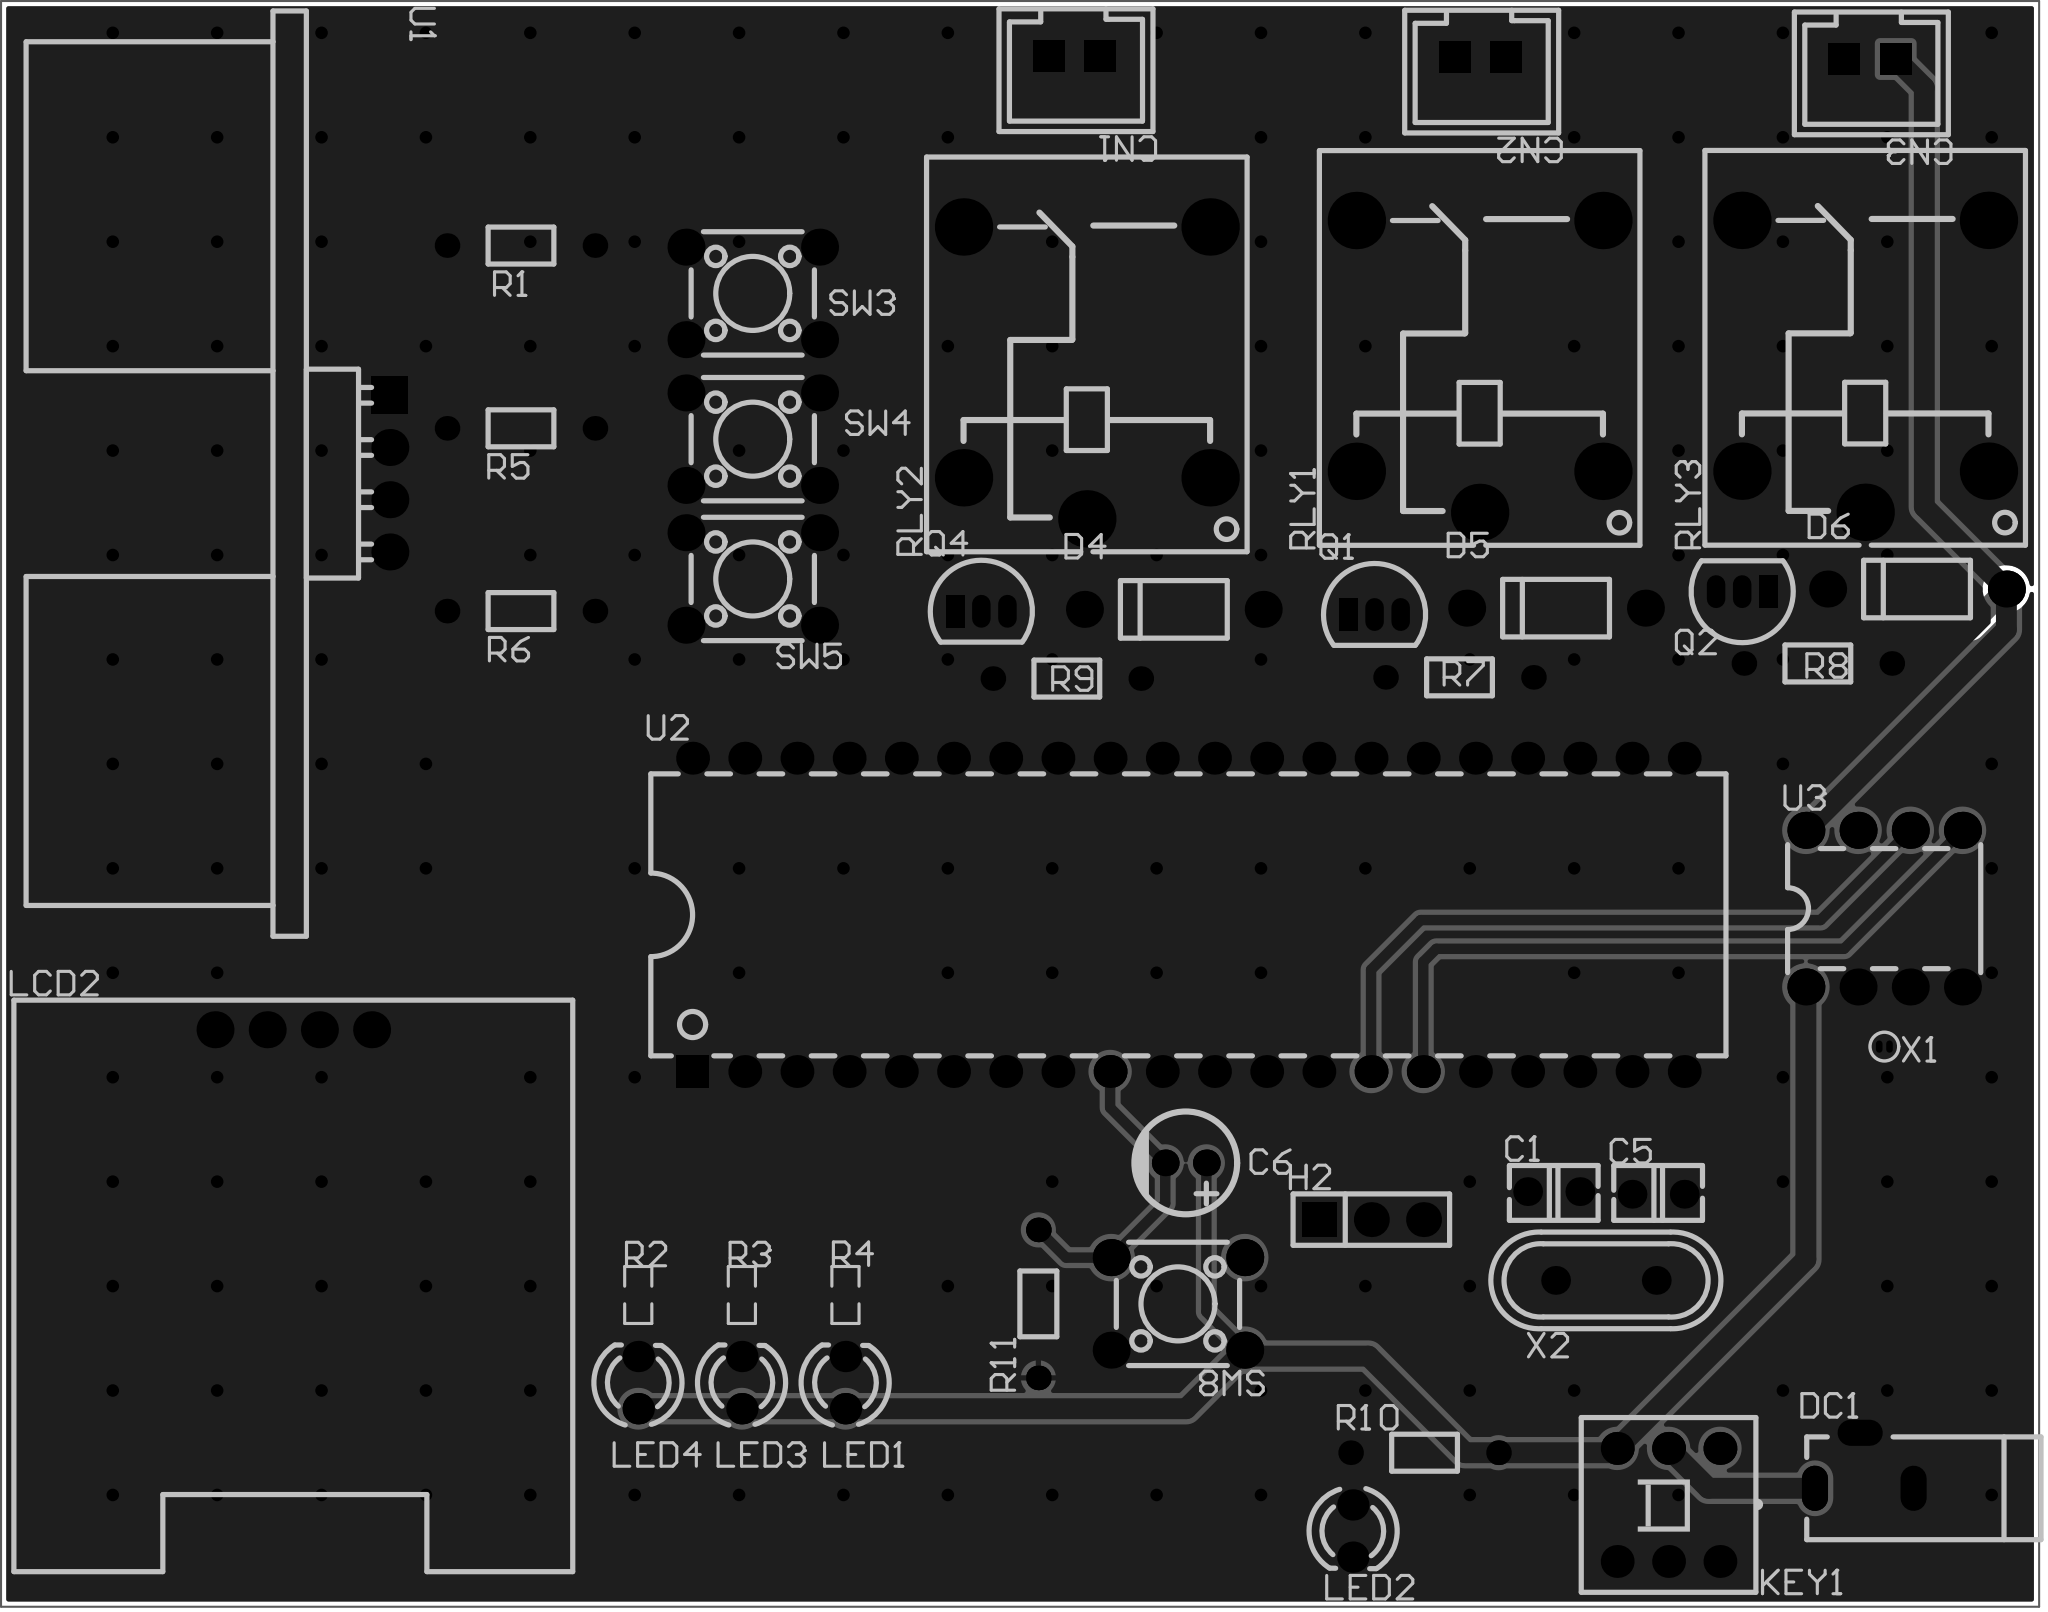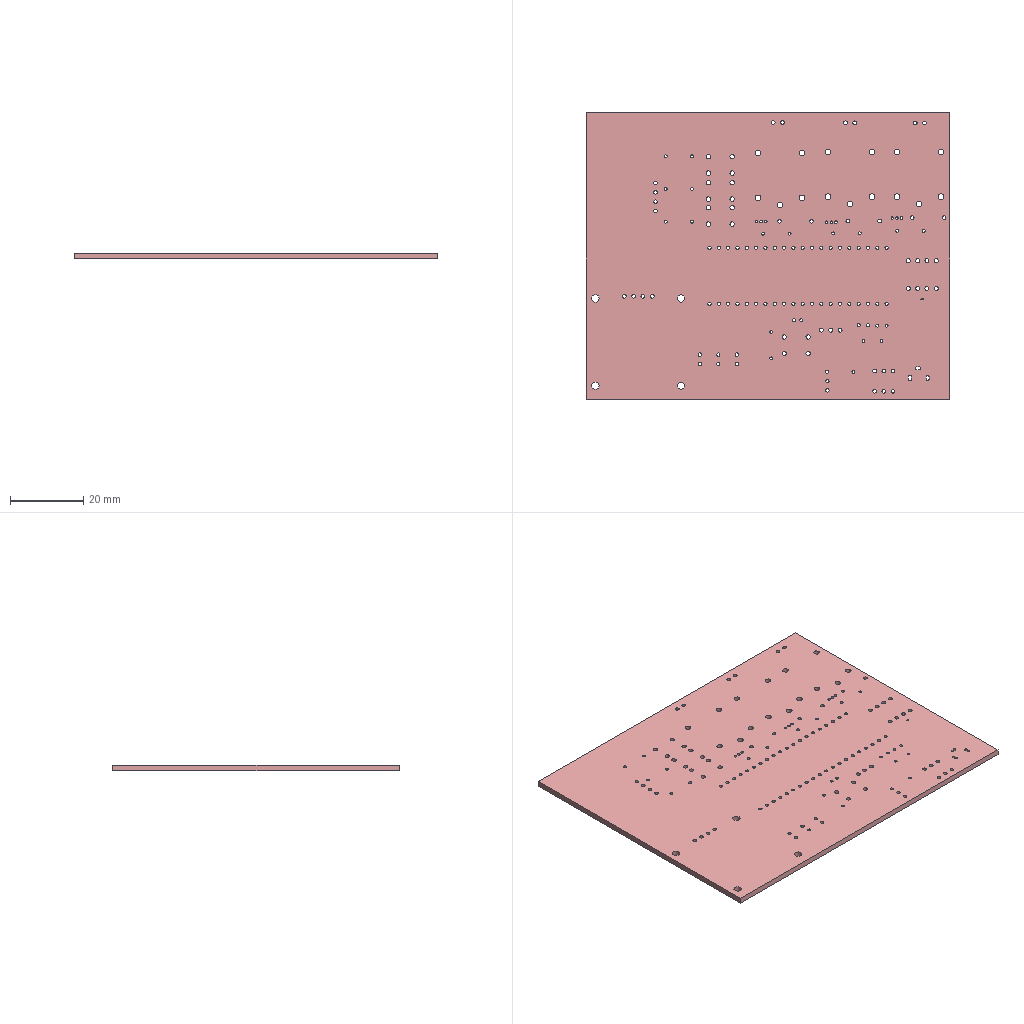Circuit board layout | Altium Designer | box 99.2 x 78.1 x 1.6 mm
Layer stack:
# Altium Designer layer stack of  (unit mm; dielectric type: 0 none, 1 core, 2 prepreg, 3 surface material)
index,name,kind,layer,copper_thickness_mm,dielectric_type,dielectric_thickness_mm,dielectric_material,dielectric_constant
0,Top Paste Mask Layer,other,,,,,,
1,Top Silkscreen Layer,other,,,,,,
2,Top Solder Mask Layer,dielectric,,,3,0.01,,3.3
3,Top Layer,copper,Top Layer,0.035,,,,
4,Dielectric1,dielectric,,,3,1.51,FR4,4.5
5,Bottom Layer,copper,Bottom Layer,0.035,,,,
6,Bottom Solder Mask Layer,dielectric,,,3,0.01,,3.3
7,Bottom Silkscreen Layer,other,,,,,,
8,Bottom Paste Mask Layer,other,,,,,,
# drill layer pairs: low layer,high layer
drill_pair,Top Layer,Bottom Layer
Part placement:
Designator,Comment,Layer,Footprint,Center-X(mm),Center-Y(mm),Rotation
C1,30pF,TopLayer,CAP-TH_L3.8-W2.5-P2.54-D0.50,161.671,110.49,0
C5,30pF,TopLayer,CAP-TH_L3.8-W2.5-P2.54-D0.50,166.751,110.363,180
CN1,XH2.54-2PIN-直针,TopLayer,CONN-TH_XH2.54-2P,138.356,165.735,180
CN2,XH2.54-2PIN-直针,TopLayer,CONN-TH_XH2.54-2P,158.101,165.668,180
CN3,XH2.54-2PIN-直针,TopLayer,CONN-TH_XH2.54-2P,177.064,165.582,180
D4,,TopLayer,DO_1N4007,143.182,138.811,0
D5,,TopLayer,DO_1N4007,161.784,138.871,0
D6,,TopLayer,DO_1N4007,179.35,139.8,0
DC1,DC-002,TopLayer,DC-IN-TH_DC-3510,176.784,97.409,0
H2,,TopLayer,HDR-TH_3P-P2.54-V-M,152.794,109.128,0
KEY1,无自锁开关 8.5×8.5 无声,TopLayer,SW-TH_6P-L8.5-W8.5-P2.54,167.259,95.25,180
LCD2,HS96L03W2C03,TopLayer,OLED-TH_L27.8-W27.2-P2.54_C9900033791,100.33,118.364,0
LED2,,TopLayer,LED_TH-3mm,151.892,93.98,270
Q1,,TopLayer,S8550P_TO-92,152.952,138.561,0
Q2,,TopLayer,S8550P_TO-92,170.841,139.673,180
Q4,,TopLayer,S8550P_TO-92,133.814,138.718,0
R1,10kΩ,TopLayer,Res_1/8W,111.41,156.507,180
R2,220,TopLayer,R0603,117.117,105.462,90
R3,220,TopLayer,R0603,122.159,105.462,90
R4,220,TopLayer,R0603,127.201,105.462,90
R5,10kΩ,TopLayer,Res_1/8W,111.41,147.618,180
R6,10kΩ,TopLayer,Res_1/8W,111.41,138.727,180
R7,1kΩ,TopLayer,Res_1/8W,157.084,135.505,0
R8,1kΩ,TopLayer,Res_1/8W,174.524,136.18,0
R9,1kΩ,TopLayer,Res_1/8W,137.975,135.445,0
R10,1kΩ,TopLayer,Res_1/8W,155.384,97.79,0
RLY1,SRD-05VDC-SL-C,TopLayer,RELAY-TH_SRD-XXVDC-XL-C,158.065,150.626,90
RLY2,SRD-05VDC-SL-C,TopLayer,RELAY-TH_SRD-XXVDC-XL-C,138.948,150.313,90
RLY3,SRD-05VDC-SL-C,TopLayer,RELAY-TH_SRD-XXVDC-XL-C,176.828,150.633,90
SW3,,TopLayer,SW-TH_4P-L6.0-W6.0-P4.50-LS6.5,122.69,154.18,180
SW4,,TopLayer,SW-TH_4P-L6.0-W6.0-P4.50-LS6.5,122.69,147.09,180
SW5,,TopLayer,SW-TH_4P-L6.0-W6.0-P4.50-LS6.5,122.69,140.291,180
U1,HC-SR04,TopLayer,TH_HC-SR04V,105.029,145.415,270
U2,STC89C52RC-40I-PDIP40,TopLayer,DIP-40_L52.0-W13.7-P2.54-LS15.2-BL,143.891,123.952,0
U3,DS1302N(XBLW),TopLayer,PDIP-8_L9.3-W6.4-P2.54-LS7.6-BL,177.752,124.254,0
X1,32.768kHz,TopLayer,CRYSTAL-TH_BD1.4-P0.45-D0.2,177.761,117.544,180
X2,11.059MHz,TopLayer,OSC-TH_L11.1-W4.7-P4.88,164.211,106.172,180
C6,10uF,TopLayer,CAP-TH_BD5.0-P2.00-D0.8-FD-10UF50VC110GL,143.764,111.887,180
R11,10kΩ,TopLayer,Res_1/8W,136.589,105.029,90
SW8,,TopLayer,SW-TH_4P-L6.0-W6.0-P4.50-LS6.5,143.383,105.029,180
LED1,,TopLayer,LED_TH-3mm,127.201,101.2,90
LED3,,TopLayer,LED_TH-3mm,122.159,101.2,90
LED4,,TopLayer,LED_TH-3mm,117.117,101.2,90
Pad and via stacks:
# Altium Designer via and pad stacks of  (unit mm). Each distinct definition once, with the count of objects using it.
# via: kind,start_layer,end_layer,hole_mm,diameter_mm,mode(0 simple;1 top-mid-bottom;2 full stack),diameter_per_layer,count,example_net
# pad: kind,layer,hole_mm,hole_type(0 round;1 square;2 slot),plating,top_size,top_shape(1 round;2 rect;3 octagon;9 rounded rect),mid_size,bottom_size,mode,footprint,size_per_layer,count,example
pad,Multi-Layer,0.8,0,plated,1.4x1.4,1,1.4x1.4,1.4x1.4,0,CAP-TH_L3.8-W2.5-P2.54-D0.50,,4,C1.1
pad,Multi-Layer,1,2,plated,1.524x1.524,2,1.524x1.524,1.524x1.524,0,CONN-TH_XH2.54-2P,,6,CN1.1
pad,Multi-Layer,1,0,plated,1.8x1.8,1,1.8x1.8,1.8x1.8,0,DO_1N4007,,6,D4.1
pad,Multi-Layer,0.8,2,plated,2.2x1.27,1,2.2x1.27,2.2x1.27,0,DC-IN-TH_DC-3510,,3,DC1.3
pad,Multi-Layer,1.1,0,plated,1.7x1.7,2,1.7x1.7,1.7x1.7,0,HDR-TH_3P-P2.54-V-M,,1,H2.1
pad,Multi-Layer,1.1,0,plated,1.7x1.7,1,1.7x1.7,1.7x1.7,0,HDR-TH_3P-P2.54-V-M,,2,H2.2
pad,Multi-Layer,1,0,plated,1.6x1.6,1,1.6x1.6,1.6x1.6,0,SW-TH_6P-L8.5-W8.5-P2.54,,6,KEY1.4
pad,Multi-Layer,1.05,0,plated,1.8x1.8,1,1.8x1.8,1.8x1.8,0,OLED-TH_L27.8-W27.2-P2.54_C9900033791,,4,LCD2.1
pad,Multi-Layer,0.9144,0,plated,1.524x1.524,1,1.524x1.524,1.524x1.524,0,LED_TH-3mm,,8,LED2.1
pad,Multi-Layer,0.7,0,plated,0.9x1.6,1,0.9x1.6,0.9x1.6,0,S8550P_TO-92,,6,Q1.3
pad,Multi-Layer,0.7,0,plated,0.9x1.6,2,0.9x1.6,0.9x1.6,0,S8550P_TO-92,,3,Q1.1
pad,Multi-Layer,0.8001,0,plated,1.199x1.199,1,1.199x1.199,1.199x1.199,0,Res_1/8W,,16,R1.1
pad,Multi-Layer,1.524,0,plated,2.794x2.794,1,2.794x2.794,2.794x2.794,0,RELAY-TH_SRD-XXVDC-XL-C,,15,RLY1.2
pad,Multi-Layer,1.2,0,plated,1.8x1.8,1,1.8x1.8,1.8x1.8,0,SW-TH_4P-L6.0-W6.0-P4.50-LS6.5,,16,SW3.1
pad,Multi-Layer,1.001,0,plated,1.8x1.8,1,1.8x1.8,1.8x1.8,0,TH_HC-SR04V,,3,U1.4
pad,Multi-Layer,1.001,0,plated,1.8x1.8,2,1.8x1.8,1.8x1.8,0,TH_HC-SR04V,,1,U1.1
pad,Multi-Layer,0.889,0,plated,1.6x1.6,1,1.6x1.6,1.6x1.6,0,DIP-40_L52.0-W13.7-P2.54-LS15.2-BL,,39,U2.31
pad,Multi-Layer,0.889,0,plated,1.6x1.6,2,1.6x1.6,1.6x1.6,0,DIP-40_L52.0-W13.7-P2.54-LS15.2-BL,,1,U2.1
pad,Multi-Layer,1.1,0,plated,1.8x1.8,1,1.8x1.8,1.8x1.8,0,PDIP-8_L9.3-W6.4-P2.54-LS7.6-BL,,8,U3.1
pad,Multi-Layer,0.27,0,plated,0.32x0.6,1,0.32x0.6,0.32x0.6,0,CRYSTAL-TH_BD1.4-P0.45-D0.2,,2,X1.1
pad,Multi-Layer,0.7,0,plated,1.4x1.4,1,1.4x1.4,1.4x1.4,0,OSC-TH_L11.1-W4.7-P4.88,,2,X2.1
pad,Multi-Layer,0.8,0,plated,1.3x1.3,1,1.3x1.3,1.3x1.3,0,CAP-TH_BD5.0-P2.00-D0.8-FD-10UF50VC110GL,,2,C6.2
pad,Top Layer,0,0,plated,0.8065x0.864,2,0.8065x0.864,0.8065x0.864,0,R0603,,6,R2.2
via,Top Layer,Bottom Layer,0.3048,0.61,0,,187,GND
Copper pours:
name,layer,net,type(0 solid;1 hatched;2 none)
Top Layer-GND,Top Layer,GND,0
Bottom Layer-GND,Bottom Layer,GND,0
Design rules, without the lines most boards share:
# Altium Designer design rules of  (exported by Altium Designer, unit mm)
# columns: name | kind | enabled | priority | scope1 | scope2 | descriptor | typed fields (field=value)
creepage | 65 | enabled | 1 | All | All | Creepage Distance Constraint =(0mil) (All),(All) |